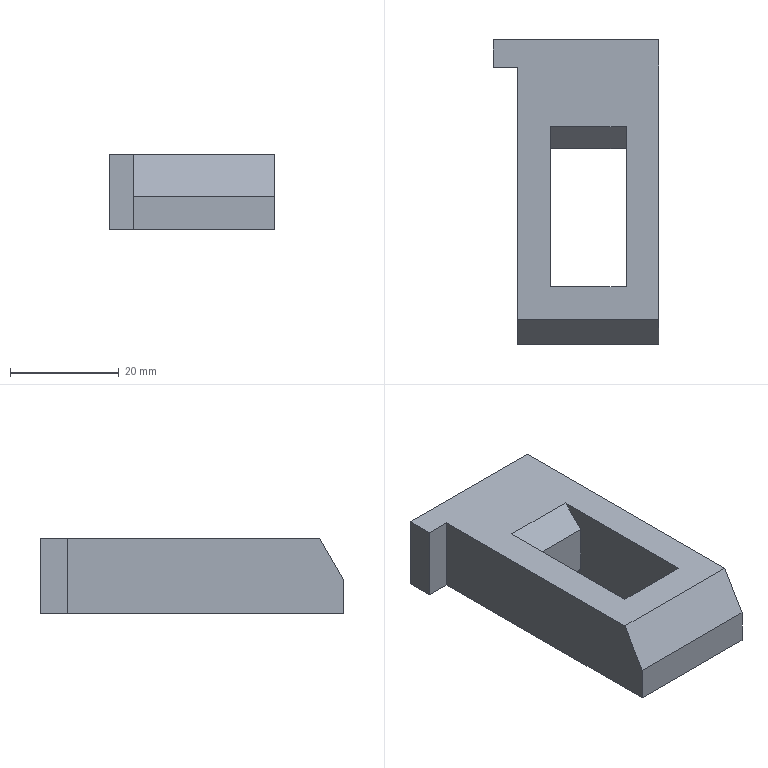Part | STEP file | solid 87 | 1 solid | 17 faces | box 30.5 x 56 x 14 mm | volume 14654 mm3 | plane 16 | cylinder 1 | commonest cylinder face diameters 11 x1